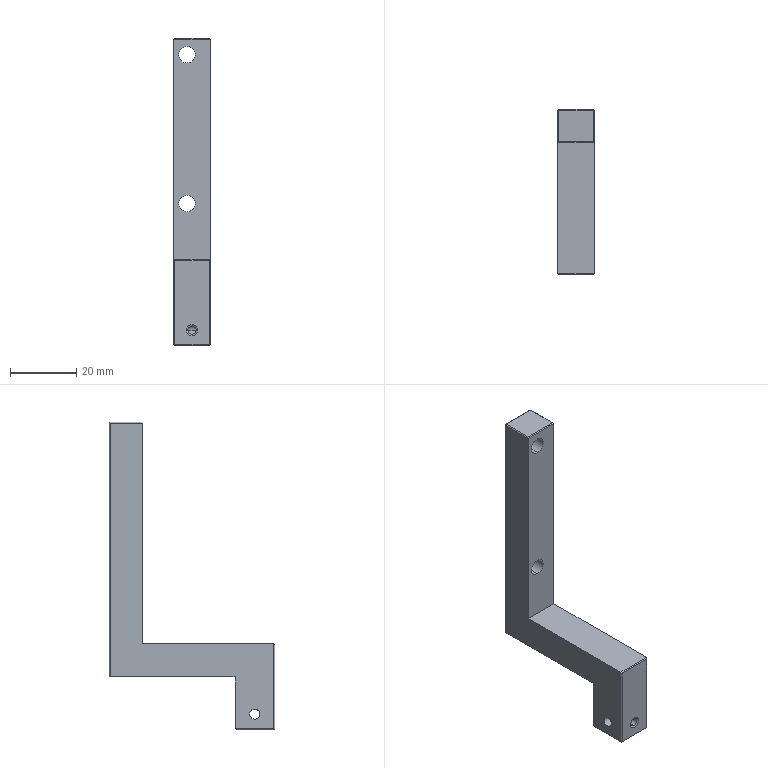Part | NX | 1 solid | 37 faces | box 11 x 50 x 93 mm | volume 14468 mm3 | plane 23 | cylinder 8 | cone 6 | commonest cylinder face diameters 5 x4 2.5 x2 3.1 x2